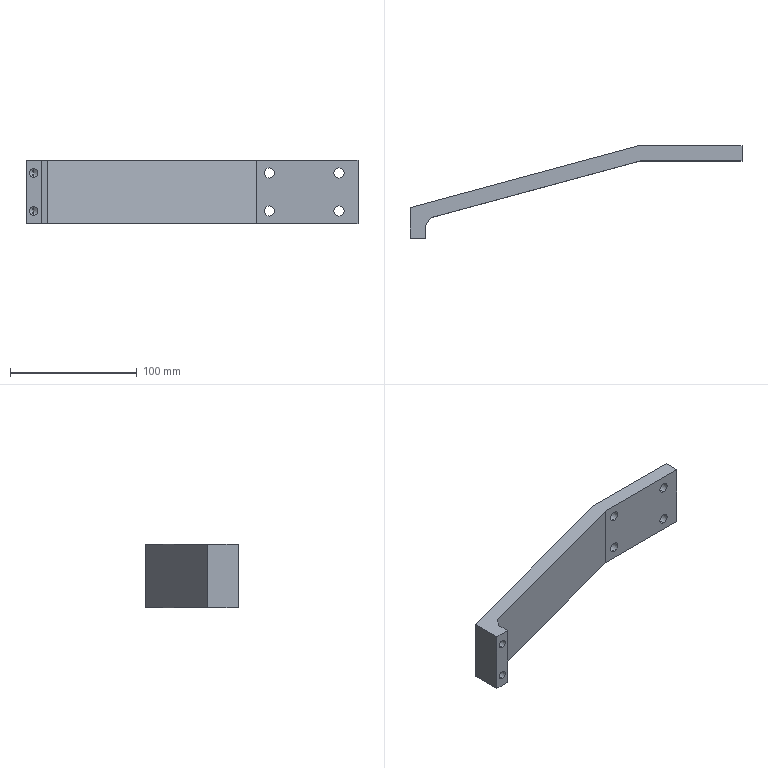Part | SolidWorks | features BaseBody 1 | 1 solid | 27 faces | box 262 x 73 x 50 mm | volume 166333 mm3 | cylinder 12 | plane 11 | cone 4 | commonest cylinder face diameters 8 x8 6.8 x4
STEP:
#1=CARTESIAN_POINT('',(260.,-92.,-78.879));
#2=VERTEX_POINT('',#1);
#3=CARTESIAN_POINT('',(260.,-92.,-86.879));
#4=VERTEX_POINT('',#3);
#5=CARTESIAN_POINT('',(260.,-92.,-82.879));
#6=DIRECTION('',(0.,-1.,0.));
#7=DIRECTION('',(0.,0.,1.));
#8=AXIS2_PLACEMENT_3D('',#5,#6,#7);
#9=CIRCLE('',#8,4.);
#10=EDGE_CURVE('',#2,#4,#9,.T.);
#11=ORIENTED_EDGE('',*,*,#10,.T.);
#12=CARTESIAN_POINT('',(260.,-80.,-86.879));
#13=VERTEX_POINT('',#12);
#14=CARTESIAN_POINT('',(260.,-153.,-86.879));
#15=DIRECTION('',(0.,1.,0.));
#16=VECTOR('',#15,1000.);
#17=LINE('',#14,#16);
#18=EDGE_CURVE('',#4,#13,#17,.T.);
#19=ORIENTED_EDGE('',*,*,#18,.T.);
#20=CARTESIAN_POINT('',(260.,-80.,-78.879));
#21=VERTEX_POINT('',#20);
#22=CARTESIAN_POINT('',(260.,-80.,-82.879));
#23=DIRECTION('',(0.,1.,0.));
#24=DIRECTION('',(0.,0.,1.));
#25=AXIS2_PLACEMENT_3D('',#22,#23,#24);
#26=CIRCLE('',#25,4.);
#27=EDGE_CURVE('',#13,#21,#26,.T.);
#28=ORIENTED_EDGE('',*,*,#27,.T.);
#29=CARTESIAN_POINT('',(260.,-153.,-78.879));
#30=DIRECTION('',(0.,1.,0.));
#31=VECTOR('',#30,1000.);
#32=LINE('',#29,#31);
#33=EDGE_CURVE('',#2,#21,#32,.T.);
#34=ORIENTED_EDGE('',*,*,#33,.F.);
#35=EDGE_LOOP('',(#11,#19,#28,#34));
#36=FACE_OUTER_BOUND('',#35,.T.);
#37=CARTESIAN_POINT('',(260.,-153.,-82.879));
#38=DIRECTION('',(0.,1.,0.));
#39=DIRECTION('',(0.,0.,1.));
#40=AXIS2_PLACEMENT_3D('',#37,#38,#39);
#41=CYLINDRICAL_SURFACE('',#40,4.);
#42=ADVANCED_FACE('',(#36),#41,.F.);
#43=CARTESIAN_POINT('',(260.,-92.,-48.879));
#44=VERTEX_POINT('',#43);
#45=CARTESIAN_POINT('',(260.,-92.,-56.879));
#46=VERTEX_POINT('',#45);
#47=CARTESIAN_POINT('',(260.,-92.,-52.879));
#48=DIRECTION('',(0.,-1.,0.));
#49=DIRECTION('',(0.,0.,1.));
#50=AXIS2_PLACEMENT_3D('',#47,#48,#49);
#51=CIRCLE('',#50,4.);
#52=EDGE_CURVE('',#44,#46,#51,.T.);
#53=ORIENTED_EDGE('',*,*,#52,.T.);
#54=CARTESIAN_POINT('',(260.,-80.,-56.879));
#55=VERTEX_POINT('',#54);
#56=CARTESIAN_POINT('',(260.,-153.,-56.879));
#57=DIRECTION('',(0.,1.,0.));
#58=VECTOR('',#57,1000.);
#59=LINE('',#56,#58);
#60=EDGE_CURVE('',#46,#55,#59,.T.);
#61=ORIENTED_EDGE('',*,*,#60,.T.);
#62=CARTESIAN_POINT('',(260.,-80.,-48.879));
#63=VERTEX_POINT('',#62);
#64=CARTESIAN_POINT('',(260.,-80.,-52.879));
#65=DIRECTION('',(0.,1.,0.));
#66=DIRECTION('',(0.,0.,1.));
#67=AXIS2_PLACEMENT_3D('',#64,#65,#66);
#68=CIRCLE('',#67,4.);
#69=EDGE_CURVE('',#55,#63,#68,.T.);
#70=ORIENTED_EDGE('',*,*,#69,.T.);
#71=CARTESIAN_POINT('',(260.,-153.,-48.879));
#72=DIRECTION('',(0.,1.,0.));
#73=VECTOR('',#72,1000.);
#74=LINE('',#71,#73);
#75=EDGE_CURVE('',#44,#63,#74,.T.);
#76=ORIENTED_EDGE('',*,*,#75,.F.);
#77=EDGE_LOOP('',(#53,#61,#70,#76));
#78=FACE_OUTER_BOUND('',#77,.T.);
#79=CARTESIAN_POINT('',(260.,-153.,-52.879));
#80=DIRECTION('',(0.,1.,0.));
#81=DIRECTION('',(0.,0.,1.));
#82=AXIS2_PLACEMENT_3D('',#79,#80,#81);
#83=CYLINDRICAL_SURFACE('',#82,4.);
#84=ADVANCED_FACE('',(#78),#83,.F.);
#85=CARTESIAN_POINT('',(315.,-92.,-48.879));
#86=VERTEX_POINT('',#85);
#87=CARTESIAN_POINT('',(315.,-92.,-56.879));
#88=VERTEX_POINT('',#87);
#89=CARTESIAN_POINT('',(315.,-92.,-52.879));
#90=DIRECTION('',(0.,-1.,0.));
#91=DIRECTION('',(0.,0.,1.));
#92=AXIS2_PLACEMENT_3D('',#89,#90,#91);
#93=CIRCLE('',#92,4.);
#94=EDGE_CURVE('',#86,#88,#93,.T.);
#95=ORIENTED_EDGE('',*,*,#94,.T.);
#96=CARTESIAN_POINT('',(315.,-80.,-56.879));
#97=VERTEX_POINT('',#96);
#98=CARTESIAN_POINT('',(315.,-153.,-56.879));
#99=DIRECTION('',(0.,1.,0.));
#100=VECTOR('',#99,1000.);
#101=LINE('',#98,#100);
#102=EDGE_CURVE('',#88,#97,#101,.T.);
#103=ORIENTED_EDGE('',*,*,#102,.T.);
#104=CARTESIAN_POINT('',(315.,-80.,-48.879));
#105=VERTEX_POINT('',#104);
#106=CARTESIAN_POINT('',(315.,-80.,-52.879));
#107=DIRECTION('',(0.,1.,0.));
#108=DIRECTION('',(0.,0.,1.));
#109=AXIS2_PLACEMENT_3D('',#106,#107,#108);
#110=CIRCLE('',#109,4.);
#111=EDGE_CURVE('',#97,#105,#110,.T.);
#112=ORIENTED_EDGE('',*,*,#111,.T.);
#113=CARTESIAN_POINT('',(315.,-153.,-48.879));
#114=DIRECTION('',(0.,1.,0.));
#115=VECTOR('',#114,1000.);
#116=LINE('',#113,#115);
#117=EDGE_CURVE('',#86,#105,#116,.T.);
#118=ORIENTED_EDGE('',*,*,#117,.F.);
#119=EDGE_LOOP('',(#95,#103,#112,#118));
#120=FACE_OUTER_BOUND('',#119,.T.);
#121=CARTESIAN_POINT('',(315.,-153.,-52.879));
#122=DIRECTION('',(0.,1.,0.));
#123=DIRECTION('',(0.,0.,1.));
#124=AXIS2_PLACEMENT_3D('',#121,#122,#123);
#125=CYLINDRICAL_SURFACE('',#124,4.);
#126=ADVANCED_FACE('',(#120),#125,.F.);
#127=CARTESIAN_POINT('',(315.,-92.,-78.879));
#128=VERTEX_POINT('',#127);
#129=CARTESIAN_POINT('',(315.,-92.,-86.879));
#130=VERTEX_POINT('',#129);
#131=CARTESIAN_POINT('',(315.,-92.,-82.879));
#132=DIRECTION('',(0.,-1.,0.));
#133=DIRECTION('',(0.,0.,1.));
#134=AXIS2_PLACEMENT_3D('',#131,#132,#133);
#135=CIRCLE('',#134,4.);
#136=EDGE_CURVE('',#128,#130,#135,.T.);
#137=ORIENTED_EDGE('',*,*,#136,.T.);
#138=CARTESIAN_POINT('',(315.,-80.,-86.879));
#139=VERTEX_POINT('',#138);
#140=CARTESIAN_POINT('',(315.,-153.,-86.879));
#141=DIRECTION('',(0.,1.,0.));
#142=VECTOR('',#141,1000.);
#143=LINE('',#140,#142);
#144=EDGE_CURVE('',#130,#139,#143,.T.);
#145=ORIENTED_EDGE('',*,*,#144,.T.);
#146=CARTESIAN_POINT('',(315.,-80.,-78.879));
#147=VERTEX_POINT('',#146);
#148=CARTESIAN_POINT('',(315.,-80.,-82.879));
#149=DIRECTION('',(0.,1.,0.));
#150=DIRECTION('',(0.,0.,1.));
#151=AXIS2_PLACEMENT_3D('',#148,#149,#150);
#152=CIRCLE('',#151,4.);
#153=EDGE_CURVE('',#139,#147,#152,.T.);
#154=ORIENTED_EDGE('',*,*,#153,.T.);
#155=CARTESIAN_POINT('',(315.,-153.,-78.879));
#156=DIRECTION('',(0.,1.,0.));
#157=VECTOR('',#156,1000.);
#158=LINE('',#155,#157);
#159=EDGE_CURVE('',#128,#147,#158,.T.);
#160=ORIENTED_EDGE('',*,*,#159,.F.);
#161=EDGE_LOOP('',(#137,#145,#154,#160));
#162=FACE_OUTER_BOUND('',#161,.T.);
#163=CARTESIAN_POINT('',(315.,-153.,-82.879));
#164=DIRECTION('',(0.,1.,0.));
#165=DIRECTION('',(0.,0.,1.));
#166=AXIS2_PLACEMENT_3D('',#163,#164,#165);
#167=CYLINDRICAL_SURFACE('',#166,4.);
#168=ADVANCED_FACE('',(#162),#167,.F.);
#169=CARTESIAN_POINT('',(74.,-140.,-49.479));
#170=VERTEX_POINT('',#169);
#171=CARTESIAN_POINT('',(74.,-140.,-56.279));
#172=VERTEX_POINT('',#171);
#173=CARTESIAN_POINT('',(74.,-140.,-52.879));
#174=DIRECTION('',(0.,-1.,0.));
#175=DIRECTION('',(0.,0.,-1.));
#176=AXIS2_PLACEMENT_3D('',#173,#174,#175);
#177=CIRCLE('',#176,3.4);
#178=EDGE_CURVE('',#170,#172,#177,.T.);
#179=ORIENTED_EDGE('',*,*,#178,.F.);
#180=CARTESIAN_POINT('',(74.,-153.,-49.479));
#181=VERTEX_POINT('',#180);
#182=CARTESIAN_POINT('',(74.,-153.,-49.479));
#183=DIRECTION('',(0.,-1.,0.));
#184=VECTOR('',#183,1000.);
#185=LINE('',#182,#184);
#186=EDGE_CURVE('',#170,#181,#185,.T.);
#187=ORIENTED_EDGE('',*,*,#186,.T.);
#188=CARTESIAN_POINT('',(74.,-153.,-56.279));
#189=VERTEX_POINT('',#188);
#190=CARTESIAN_POINT('',(74.,-153.,-52.879));
#191=DIRECTION('',(0.,-1.,0.));
#192=DIRECTION('',(0.,0.,-1.));
#193=AXIS2_PLACEMENT_3D('',#190,#191,#192);
#194=CIRCLE('',#193,3.4);
#195=EDGE_CURVE('',#181,#189,#194,.T.);
#196=ORIENTED_EDGE('',*,*,#195,.T.);
#197=CARTESIAN_POINT('',(74.,-153.,-56.279));
#198=DIRECTION('',(0.,-1.,0.));
#199=VECTOR('',#198,1000.);
#200=LINE('',#197,#199);
#201=EDGE_CURVE('',#172,#189,#200,.T.);
#202=ORIENTED_EDGE('',*,*,#201,.F.);
#203=EDGE_LOOP('',(#179,#187,#196,#202));
#204=FACE_OUTER_BOUND('',#203,.T.);
#205=CARTESIAN_POINT('',(74.,-153.,-52.879));
#206=DIRECTION('',(0.,-1.,0.));
#207=DIRECTION('',(0.,0.,-1.));
#208=AXIS2_PLACEMENT_3D('',#205,#206,#207);
#209=CYLINDRICAL_SURFACE('',#208,3.4);
#210=ADVANCED_FACE('',(#204),#209,.F.);
#211=CARTESIAN_POINT('',(74.,-140.,-79.479));
#212=VERTEX_POINT('',#211);
#213=CARTESIAN_POINT('',(74.,-140.,-86.279));
#214=VERTEX_POINT('',#213);
#215=CARTESIAN_POINT('',(74.,-140.,-82.879));
#216=DIRECTION('',(0.,-1.,0.));
#217=DIRECTION('',(0.,0.,-1.));
#218=AXIS2_PLACEMENT_3D('',#215,#216,#217);
#219=CIRCLE('',#218,3.4);
#220=EDGE_CURVE('',#212,#214,#219,.T.);
#221=ORIENTED_EDGE('',*,*,#220,.F.);
#222=CARTESIAN_POINT('',(74.,-153.,-79.479));
#223=VERTEX_POINT('',#222);
#224=CARTESIAN_POINT('',(74.,-153.,-79.479));
#225=DIRECTION('',(0.,-1.,0.));
#226=VECTOR('',#225,1000.);
#227=LINE('',#224,#226);
#228=EDGE_CURVE('',#212,#223,#227,.T.);
#229=ORIENTED_EDGE('',*,*,#228,.T.);
#230=CARTESIAN_POINT('',(74.,-153.,-86.279));
#231=VERTEX_POINT('',#230);
#232=CARTESIAN_POINT('',(74.,-153.,-82.879));
#233=DIRECTION('',(0.,-1.,0.));
#234=DIRECTION('',(0.,0.,-1.));
#235=AXIS2_PLACEMENT_3D('',#232,#233,#234);
#236=CIRCLE('',#235,3.4);
#237=EDGE_CURVE('',#223,#231,#236,.T.);
#238=ORIENTED_EDGE('',*,*,#237,.T.);
#239=CARTESIAN_POINT('',(74.,-153.,-86.279));
#240=DIRECTION('',(0.,-1.,0.));
#241=VECTOR('',#240,1000.);
#242=LINE('',#239,#241);
#243=EDGE_CURVE('',#214,#231,#242,.T.);
#244=ORIENTED_EDGE('',*,*,#243,.F.);
#245=EDGE_LOOP('',(#221,#229,#238,#244));
#246=FACE_OUTER_BOUND('',#245,.T.);
#247=CARTESIAN_POINT('',(74.,-153.,-82.879));
#248=DIRECTION('',(0.,-1.,0.));
#249=DIRECTION('',(0.,0.,-1.));
#250=AXIS2_PLACEMENT_3D('',#247,#248,#249);
#251=CYLINDRICAL_SURFACE('',#250,3.4);
#252=ADVANCED_FACE('',(#246),#251,.F.);
#253=CARTESIAN_POINT('',(74.,-137.957,-52.879));
#254=VERTEX_POINT('',#253);
#255=CARTESIAN_POINT('',(74.,-140.,-56.279));
#256=DIRECTION('',(0.,-0.515,-0.8572));
#257=VECTOR('',#256,1000.);
#258=LINE('',#255,#257);
#259=EDGE_CURVE('',#254,#172,#258,.T.);
#260=ORIENTED_EDGE('',*,*,#259,.F.);
#261=CARTESIAN_POINT('',(74.,-140.,-49.479));
#262=DIRECTION('',(0.,-0.515,0.8572));
#263=VECTOR('',#262,1000.);
#264=LINE('',#261,#263);
#265=EDGE_CURVE('',#254,#170,#264,.T.);
#266=ORIENTED_EDGE('',*,*,#265,.T.);
#267=ORIENTED_EDGE('',*,*,#178,.T.);
#268=EDGE_LOOP('',(#260,#266,#267));
#269=FACE_OUTER_BOUND('',#268,.T.);
#270=CARTESIAN_POINT('',(74.,-140.,-52.879));
#271=DIRECTION('',(0.,-1.,0.));
#272=DIRECTION('',(0.,0.,-1.));
#273=AXIS2_PLACEMENT_3D('',#270,#271,#272);
#274=CONICAL_SURFACE('',#273,3.4,1.03);
#275=ADVANCED_FACE('',(#269),#274,.F.);
#276=CARTESIAN_POINT('',(74.,-137.957,-82.879));
#277=VERTEX_POINT('',#276);
#278=CARTESIAN_POINT('',(74.,-140.,-86.279));
#279=DIRECTION('',(0.,-0.515,-0.8572));
#280=VECTOR('',#279,1000.);
#281=LINE('',#278,#280);
#282=EDGE_CURVE('',#277,#214,#281,.T.);
#283=ORIENTED_EDGE('',*,*,#282,.F.);
#284=CARTESIAN_POINT('',(74.,-140.,-79.479));
#285=DIRECTION('',(0.,-0.515,0.8572));
#286=VECTOR('',#285,1000.);
#287=LINE('',#284,#286);
#288=EDGE_CURVE('',#277,#212,#287,.T.);
#289=ORIENTED_EDGE('',*,*,#288,.T.);
#290=ORIENTED_EDGE('',*,*,#220,.T.);
#291=EDGE_LOOP('',(#283,#289,#290));
#292=FACE_OUTER_BOUND('',#291,.T.);
#293=CARTESIAN_POINT('',(74.,-140.,-82.879));
#294=DIRECTION('',(0.,-1.,0.));
#295=DIRECTION('',(0.,0.,-1.));
#296=AXIS2_PLACEMENT_3D('',#293,#294,#295);
#297=CONICAL_SURFACE('',#296,3.4,1.03);
#298=ADVANCED_FACE('',(#292),#297,.F.);
#299=CARTESIAN_POINT('',(248.405,-80.,-92.879));
#300=VERTEX_POINT('',#299);
#301=CARTESIAN_POINT('',(248.405,-80.,-42.879));
#302=VERTEX_POINT('',#301);
#303=CARTESIAN_POINT('',(248.405,-80.,-92.879));
#304=DIRECTION('',(0.,0.,1.));
#305=VECTOR('',#304,1000.);
#306=LINE('',#303,#305);
#307=EDGE_CURVE('',#300,#302,#306,.T.);
#308=ORIENTED_EDGE('',*,*,#307,.F.);
#309=CARTESIAN_POINT('',(68.,-128.816,-92.879));
#310=VERTEX_POINT('',#309);
#311=CARTESIAN_POINT('',(68.,-128.816,-92.879));
#312=DIRECTION('',(0.9653,0.2612,0.));
#313=VECTOR('',#312,1000.);
#314=LINE('',#311,#313);
#315=EDGE_CURVE('',#310,#300,#314,.T.);
#316=ORIENTED_EDGE('',*,*,#315,.F.);
#317=CARTESIAN_POINT('',(68.,-128.816,-42.879));
#318=VERTEX_POINT('',#317);
#319=CARTESIAN_POINT('',(68.,-128.816,-92.879));
#320=DIRECTION('',(0.,0.,-1.));
#321=VECTOR('',#320,1000.);
#322=LINE('',#319,#321);
#323=EDGE_CURVE('',#318,#310,#322,.T.);
#324=ORIENTED_EDGE('',*,*,#323,.F.);
#325=CARTESIAN_POINT('',(68.,-128.816,-42.879));
#326=DIRECTION('',(-0.9653,-0.2612,0.));
#327=VECTOR('',#326,1000.);
#328=LINE('',#325,#327);
#329=EDGE_CURVE('',#302,#318,#328,.T.);
#330=ORIENTED_EDGE('',*,*,#329,.F.);
#331=EDGE_LOOP('',(#308,#316,#324,#330));
#332=FACE_OUTER_BOUND('',#331,.T.);
#333=CARTESIAN_POINT('',(68.,-128.816,-92.879));
#334=DIRECTION('',(0.2612,-0.9653,0.));
#335=DIRECTION('',(0.9653,0.2612,0.));
#336=AXIS2_PLACEMENT_3D('',#333,#334,#335);
#337=PLANE('',#336);
#338=ADVANCED_FACE('',(#332),#337,.F.);
#339=CARTESIAN_POINT('',(80.,-143.,-42.879));
#340=VERTEX_POINT('',#339);
#341=CARTESIAN_POINT('',(80.,-153.,-42.879));
#342=VERTEX_POINT('',#341);
#343=CARTESIAN_POINT('',(80.,-108.6,-42.879));
#344=DIRECTION('',(0.,-1.,0.));
#345=VECTOR('',#344,1000.);
#346=LINE('',#343,#345);
#347=EDGE_CURVE('',#340,#342,#346,.T.);
#348=ORIENTED_EDGE('',*,*,#347,.F.);
#349=CARTESIAN_POINT('',(84.826,-136.694,-42.879));
#350=VERTEX_POINT('',#349);
#351=CARTESIAN_POINT('',(84.826,-136.694,-42.879));
#352=DIRECTION('',(-0.6078,-0.7941,0.));
#353=VECTOR('',#352,1000.);
#354=LINE('',#351,#353);
#355=EDGE_CURVE('',#350,#340,#354,.T.);
#356=ORIENTED_EDGE('',*,*,#355,.F.);
#357=CARTESIAN_POINT('',(250.,-92.,-42.879));
#358=VERTEX_POINT('',#357);
#359=CARTESIAN_POINT('',(250.,-92.,-42.879));
#360=DIRECTION('',(-0.9653,-0.2612,0.));
#361=VECTOR('',#360,1000.);
#362=LINE('',#359,#361);
#363=EDGE_CURVE('',#358,#350,#362,.T.);
#364=ORIENTED_EDGE('',*,*,#363,.F.);
#365=CARTESIAN_POINT('',(330.,-92.,-42.879));
#366=VERTEX_POINT('',#365);
#367=CARTESIAN_POINT('',(68.,-92.,-42.879));
#368=DIRECTION('',(-1.,0.,0.));
#369=VECTOR('',#368,1000.);
#370=LINE('',#367,#369);
#371=EDGE_CURVE('',#366,#358,#370,.T.);
#372=ORIENTED_EDGE('',*,*,#371,.F.);
#373=CARTESIAN_POINT('',(330.,-80.,-42.879));
#374=VERTEX_POINT('',#373);
#375=CARTESIAN_POINT('',(330.,-108.6,-42.879));
#376=DIRECTION('',(0.,-1.,0.));
#377=VECTOR('',#376,1000.);
#378=LINE('',#375,#377);
#379=EDGE_CURVE('',#374,#366,#378,.T.);
#380=ORIENTED_EDGE('',*,*,#379,.F.);
#381=CARTESIAN_POINT('',(68.,-80.,-42.879));
#382=DIRECTION('',(1.,0.,0.));
#383=VECTOR('',#382,1000.);
#384=LINE('',#381,#383);
#385=EDGE_CURVE('',#302,#374,#384,.T.);
#386=ORIENTED_EDGE('',*,*,#385,.F.);
#387=ORIENTED_EDGE('',*,*,#329,.T.);
#388=CARTESIAN_POINT('',(68.,-153.,-42.879));
#389=VERTEX_POINT('',#388);
#390=CARTESIAN_POINT('',(68.,-108.6,-42.879));
#391=DIRECTION('',(0.,1.,0.));
#392=VECTOR('',#391,1000.);
#393=LINE('',#390,#392);
#394=EDGE_CURVE('',#389,#318,#393,.T.);
#395=ORIENTED_EDGE('',*,*,#394,.F.);
#396=CARTESIAN_POINT('',(68.,-153.,-42.879));
#397=DIRECTION('',(-1.,0.,0.));
#398=VECTOR('',#397,1000.);
#399=LINE('',#396,#398);
#400=EDGE_CURVE('',#342,#389,#399,.T.);
#401=ORIENTED_EDGE('',*,*,#400,.F.);
#402=EDGE_LOOP('',(#348,#356,#364,#372,#380,#386,#387,#395,#401));
#403=FACE_OUTER_BOUND('',#402,.T.);
#404=CARTESIAN_POINT('',(68.,-108.6,-42.879));
#405=DIRECTION('',(0.,0.,-1.));
#406=DIRECTION('',(-1.,0.,0.));
#407=AXIS2_PLACEMENT_3D('',#404,#405,#406);
#408=PLANE('',#407);
#409=ADVANCED_FACE('',(#403),#408,.F.);
#410=CARTESIAN_POINT('',(330.,-80.,-92.879));
#411=VERTEX_POINT('',#410);
#412=CARTESIAN_POINT('',(330.,-80.,-92.879));
#413=DIRECTION('',(0.,0.,1.));
#414=VECTOR('',#413,1000.);
#415=LINE('',#412,#414);
#416=EDGE_CURVE('',#411,#374,#415,.T.);
#417=ORIENTED_EDGE('',*,*,#416,.F.);
#418=CARTESIAN_POINT('',(248.405,-80.,-92.879));
#419=DIRECTION('',(1.,0.,0.));
#420=VECTOR('',#419,1000.);
#421=LINE('',#418,#420);
#422=EDGE_CURVE('',#300,#411,#421,.T.);
#423=ORIENTED_EDGE('',*,*,#422,.F.);
#424=ORIENTED_EDGE('',*,*,#307,.T.);
#425=ORIENTED_EDGE('',*,*,#385,.T.);
#426=EDGE_LOOP('',(#417,#423,#424,#425));
#427=FACE_OUTER_BOUND('',#426,.T.);
#428=CARTESIAN_POINT('',(260.,-80.,-82.879));
#429=DIRECTION('',(0.,1.,0.));
#430=DIRECTION('',(0.,0.,1.));
#431=AXIS2_PLACEMENT_3D('',#428,#429,#430);
#432=CIRCLE('',#431,4.);
#433=EDGE_CURVE('',#21,#13,#432,.T.);
#434=ORIENTED_EDGE('',*,*,#433,.F.);
#435=ORIENTED_EDGE('',*,*,#27,.F.);
#436=EDGE_LOOP('',(#434,#435));
#437=FACE_BOUND('',#436,.T.);
#438=CARTESIAN_POINT('',(260.,-80.,-52.879));
#439=DIRECTION('',(0.,1.,0.));
#440=DIRECTION('',(0.,0.,1.));
#441=AXIS2_PLACEMENT_3D('',#438,#439,#440);
#442=CIRCLE('',#441,4.);
#443=EDGE_CURVE('',#63,#55,#442,.T.);
#444=ORIENTED_EDGE('',*,*,#443,.F.);
#445=ORIENTED_EDGE('',*,*,#69,.F.);
#446=EDGE_LOOP('',(#444,#445));
#447=FACE_BOUND('',#446,.T.);
#448=CARTESIAN_POINT('',(315.,-80.,-52.879));
#449=DIRECTION('',(0.,1.,0.));
#450=DIRECTION('',(0.,0.,1.));
#451=AXIS2_PLACEMENT_3D('',#448,#449,#450);
#452=CIRCLE('',#451,4.);
#453=EDGE_CURVE('',#105,#97,#452,.T.);
#454=ORIENTED_EDGE('',*,*,#453,.F.);
#455=ORIENTED_EDGE('',*,*,#111,.F.);
#456=EDGE_LOOP('',(#454,#455));
#457=FACE_BOUND('',#456,.T.);
#458=CARTESIAN_POINT('',(315.,-80.,-82.879));
#459=DIRECTION('',(0.,1.,0.));
#460=DIRECTION('',(0.,0.,1.));
#461=AXIS2_PLACEMENT_3D('',#458,#459,#460);
#462=CIRCLE('',#461,4.);
#463=EDGE_CURVE('',#147,#139,#462,.T.);
#464=ORIENTED_EDGE('',*,*,#463,.F.);
#465=ORIENTED_EDGE('',*,*,#153,.F.);
#466=EDGE_LOOP('',(#464,#465));
#467=FACE_BOUND('',#466,.T.);
#468=CARTESIAN_POINT('',(248.405,-80.,-92.879));
#469=DIRECTION('',(0.,-1.,0.));
#470=DIRECTION('',(0.,0.,-1.));
#471=AXIS2_PLACEMENT_3D('',#468,#469,#470);
#472=PLANE('',#471);
#473=ADVANCED_FACE('',(#427,#437,#447,#457,#467),#472,.F.);
#474=CARTESIAN_POINT('',(84.826,-136.694,-92.879));
#475=VERTEX_POINT('',#474);
#476=CARTESIAN_POINT('',(80.,-143.,-92.879));
#477=VERTEX_POINT('',#476);
#478=CARTESIAN_POINT('',(84.826,-136.694,-92.879));
#479=DIRECTION('',(-0.6078,-0.7941,0.));
#480=VECTOR('',#479,1000.);
#481=LINE('',#478,#480);
#482=EDGE_CURVE('',#475,#477,#481,.T.);
#483=ORIENTED_EDGE('',*,*,#482,.T.);
#484=CARTESIAN_POINT('',(80.,-153.,-92.879));
#485=VERTEX_POINT('',#484);
#486=CARTESIAN_POINT('',(80.,-108.6,-92.879));
#487=DIRECTION('',(0.,-1.,0.));
#488=VECTOR('',#487,1000.);
#489=LINE('',#486,#488);
#490=EDGE_CURVE('',#477,#485,#489,.T.);
#491=ORIENTED_EDGE('',*,*,#490,.T.);
#492=CARTESIAN_POINT('',(68.,-153.,-92.879));
#493=VERTEX_POINT('',#492);
#494=CARTESIAN_POINT('',(68.,-153.,-92.879));
#495=DIRECTION('',(-1.,0.,0.));
#496=VECTOR('',#495,1000.);
#497=LINE('',#494,#496);
#498=EDGE_CURVE('',#485,#493,#497,.T.);
#499=ORIENTED_EDGE('',*,*,#498,.T.);
#500=CARTESIAN_POINT('',(68.,-108.6,-92.879));
#501=DIRECTION('',(0.,1.,0.));
#502=VECTOR('',#501,1000.);
#503=LINE('',#500,#502);
#504=EDGE_CURVE('',#493,#310,#503,.T.);
#505=ORIENTED_EDGE('',*,*,#504,.T.);
#506=ORIENTED_EDGE('',*,*,#315,.T.);
#507=ORIENTED_EDGE('',*,*,#422,.T.);
#508=CARTESIAN_POINT('',(330.,-92.,-92.879));
#509=VERTEX_POINT('',#508);
#510=CARTESIAN_POINT('',(330.,-108.6,-92.879));
#511=DIRECTION('',(0.,-1.,0.));
#512=VECTOR('',#511,1000.);
#513=LINE('',#510,#512);
#514=EDGE_CURVE('',#411,#509,#513,.T.);
#515=ORIENTED_EDGE('',*,*,#514,.T.);
#516=CARTESIAN_POINT('',(250.,-92.,-92.879));
#517=VERTEX_POINT('',#516);
#518=CARTESIAN_POINT('',(68.,-92.,-92.879));
#519=DIRECTION('',(-1.,0.,0.));
#520=VECTOR('',#519,1000.);
#521=LINE('',#518,#520);
#522=EDGE_CURVE('',#509,#517,#521,.T.);
#523=ORIENTED_EDGE('',*,*,#522,.T.);
#524=CARTESIAN_POINT('',(250.,-92.,-92.879));
#525=DIRECTION('',(-0.9653,-0.2612,0.));
#526=VECTOR('',#525,1000.);
#527=LINE('',#524,#526);
#528=EDGE_CURVE('',#517,#475,#527,.T.);
#529=ORIENTED_EDGE('',*,*,#528,.T.);
#530=EDGE_LOOP('',(#483,#491,#499,#505,#506,#507,#515,#523,#529));
#531=FACE_OUTER_BOUND('',#530,.T.);
#532=CARTESIAN_POINT('',(68.,-108.6,-92.879));
#533=DIRECTION('',(0.,0.,-1.));
#534=DIRECTION('',(-1.,0.,0.));
#535=AXIS2_PLACEMENT_3D('',#532,#533,#534);
#536=PLANE('',#535);
#537=ADVANCED_FACE('',(#531),#536,.T.);
#538=ORIENTED_EDGE('',*,*,#323,.T.);
#539=ORIENTED_EDGE('',*,*,#504,.F.);
#540=CARTESIAN_POINT('',(68.,-153.,-92.879));
#541=DIRECTION('',(0.,0.,-1.));
#542=VECTOR('',#541,1000.);
#543=LINE('',#540,#542);
#544=EDGE_CURVE('',#389,#493,#543,.T.);
#545=ORIENTED_EDGE('',*,*,#544,.F.);
#546=ORIENTED_EDGE('',*,*,#394,.T.);
#547=EDGE_LOOP('',(#538,#539,#545,#546));
#548=FACE_OUTER_BOUND('',#547,.T.);
#549=CARTESIAN_POINT('',(68.,-153.,-92.879));
#550=DIRECTION('',(1.,0.,0.));
#551=DIRECTION('',(0.,0.,-1.));
#552=AXIS2_PLACEMENT_3D('',#549,#550,#551);
#553=PLANE('',#552);
#554=ADVANCED_FACE('',(#548),#553,.F.);
#555=ORIENTED_EDGE('',*,*,#544,.T.);
#556=ORIENTED_EDGE('',*,*,#498,.F.);
#557=CARTESIAN_POINT('',(80.,-153.,-92.879));
#558=DIRECTION('',(0.,0.,-1.));
#559=VECTOR('',#558,1000.);
#560=LINE('',#557,#559);
#561=EDGE_CURVE('',#342,#485,#560,.T.);
#562=ORIENTED_EDGE('',*,*,#561,.F.);
#563=ORIENTED_EDGE('',*,*,#400,.T.);
#564=EDGE_LOOP('',(#555,#556,#562,#563));
#565=FACE_OUTER_BOUND('',#564,.T.);
#566=CARTESIAN_POINT('',(74.,-153.,-52.879));
#567=DIRECTION('',(0.,-1.,0.));
#568=DIRECTION('',(0.,0.,-1.));
#569=AXIS2_PLACEMENT_3D('',#566,#567,#568);
#570=CIRCLE('',#569,3.4);
#571=EDGE_CURVE('',#189,#181,#570,.T.);
#572=ORIENTED_EDGE('',*,*,#571,.F.);
#573=ORIENTED_EDGE('',*,*,#195,.F.);
#574=EDGE_LOOP('',(#572,#573));
#575=FACE_BOUND('',#574,.T.);
#576=CARTESIAN_POINT('',(74.,-153.,-82.879));
#577=DIRECTION('',(0.,-1.,0.));
#578=DIRECTION('',(0.,0.,-1.));
#579=AXIS2_PLACEMENT_3D('',#576,#577,#578);
#580=CIRCLE('',#579,3.4);
#581=EDGE_CURVE('',#231,#223,#580,.T.);
#582=ORIENTED_EDGE('',*,*,#581,.F.);
#583=ORIENTED_EDGE('',*,*,#237,.F.);
#584=EDGE_LOOP('',(#582,#583));
#585=FACE_BOUND('',#584,.T.);
#586=CARTESIAN_POINT('',(80.,-153.,-92.879));
#587=DIRECTION('',(0.,1.,0.));
#588=DIRECTION('',(0.,0.,1.));
#589=AXIS2_PLACEMENT_3D('',#586,#587,#588);
#590=PLANE('',#589);
#591=ADVANCED_FACE('',(#565,#575,#585),#590,.F.);
#592=CARTESIAN_POINT('',(80.,-143.,-92.879));
#593=DIRECTION('',(0.,0.,-1.));
#594=VECTOR('',#593,1000.);
#595=LINE('',#592,#594);
#596=EDGE_CURVE('',#340,#477,#595,.T.);
#597=ORIENTED_EDGE('',*,*,#596,.F.);
#598=ORIENTED_EDGE('',*,*,#347,.T.);
#599=ORIENTED_EDGE('',*,*,#561,.T.);
#600=ORIENTED_EDGE('',*,*,#490,.F.);
#601=EDGE_LOOP('',(#597,#598,#599,#600));
#602=FACE_OUTER_BOUND('',#601,.T.);
#603=CARTESIAN_POINT('',(80.,-153.,-92.879));
#604=DIRECTION('',(-1.,0.,0.));
#605=DIRECTION('',(0.,0.,1.));
#606=AXIS2_PLACEMENT_3D('',#603,#604,#605);
#607=PLANE('',#606);
#608=ADVANCED_FACE('',(#602),#607,.F.);
#609=ORIENTED_EDGE('',*,*,#355,.T.);
#610=ORIENTED_EDGE('',*,*,#596,.T.);
#611=ORIENTED_EDGE('',*,*,#482,.F.);
#612=CARTESIAN_POINT('',(84.826,-136.694,-92.879));
#613=DIRECTION('',(0.,0.,1.));
#614=VECTOR('',#613,1000.);
#615=LINE('',#612,#614);
#616=EDGE_CURVE('',#475,#350,#615,.T.);
#617=ORIENTED_EDGE('',*,*,#616,.T.);
#618=EDGE_LOOP('',(#609,#610,#611,#617));
#619=FACE_OUTER_BOUND('',#618,.T.);
#620=CARTESIAN_POINT('',(80.,-143.,-92.879));
#621=DIRECTION('',(0.7941,-0.6078,0.));
#622=DIRECTION('',(0.6078,0.7941,0.));
#623=AXIS2_PLACEMENT_3D('',#620,#621,#622);
#624=PLANE('',#623);
#625=ADVANCED_FACE('',(#619),#624,.T.);
#626=ORIENTED_EDGE('',*,*,#616,.F.);
#627=ORIENTED_EDGE('',*,*,#528,.F.);
#628=CARTESIAN_POINT('',(250.,-92.,-92.879));
#629=DIRECTION('',(0.,0.,-1.));
#630=VECTOR('',#629,1000.);
#631=LINE('',#628,#630);
#632=EDGE_CURVE('',#358,#517,#631,.T.);
#633=ORIENTED_EDGE('',*,*,#632,.F.);
#634=ORIENTED_EDGE('',*,*,#363,.T.);
#635=EDGE_LOOP('',(#626,#627,#633,#634));
#636=FACE_OUTER_BOUND('',#635,.T.);
#637=CARTESIAN_POINT('',(80.,-138.,-92.879));
#638=DIRECTION('',(-0.2612,0.9653,0.));
#639=DIRECTION('',(-0.9653,-0.2612,0.));
#640=AXIS2_PLACEMENT_3D('',#637,#638,#639);
#641=PLANE('',#640);
#642=ADVANCED_FACE('',(#636),#641,.F.);
#643=ORIENTED_EDGE('',*,*,#632,.T.);
#644=ORIENTED_EDGE('',*,*,#522,.F.);
#645=CARTESIAN_POINT('',(330.,-92.,-92.879));
#646=DIRECTION('',(0.,0.,-1.));
#647=VECTOR('',#646,1000.);
#648=LINE('',#645,#647);
#649=EDGE_CURVE('',#366,#509,#648,.T.);
#650=ORIENTED_EDGE('',*,*,#649,.F.);
#651=ORIENTED_EDGE('',*,*,#371,.T.);
#652=EDGE_LOOP('',(#643,#644,#650,#651));
#653=FACE_OUTER_BOUND('',#652,.T.);
#654=ORIENTED_EDGE('',*,*,#10,.F.);
#655=CARTESIAN_POINT('',(260.,-92.,-82.879));
#656=DIRECTION('',(0.,-1.,0.));
#657=DIRECTION('',(0.,0.,1.));
#658=AXIS2_PLACEMENT_3D('',#655,#656,#657);
#659=CIRCLE('',#658,4.);
#660=EDGE_CURVE('',#4,#2,#659,.T.);
#661=ORIENTED_EDGE('',*,*,#660,.F.);
#662=EDGE_LOOP('',(#654,#661));
#663=FACE_BOUND('',#662,.T.);
#664=ORIENTED_EDGE('',*,*,#52,.F.);
#665=CARTESIAN_POINT('',(260.,-92.,-52.879));
#666=DIRECTION('',(0.,-1.,0.));
#667=DIRECTION('',(0.,0.,1.));
#668=AXIS2_PLACEMENT_3D('',#665,#666,#667);
#669=CIRCLE('',#668,4.);
#670=EDGE_CURVE('',#46,#44,#669,.T.);
#671=ORIENTED_EDGE('',*,*,#670,.F.);
#672=EDGE_LOOP('',(#664,#671));
#673=FACE_BOUND('',#672,.T.);
#674=ORIENTED_EDGE('',*,*,#94,.F.);
#675=CARTESIAN_POINT('',(315.,-92.,-52.879));
#676=DIRECTION('',(0.,-1.,0.));
#677=DIRECTION('',(0.,0.,1.));
#678=AXIS2_PLACEMENT_3D('',#675,#676,#677);
#679=CIRCLE('',#678,4.);
#680=EDGE_CURVE('',#88,#86,#679,.T.);
#681=ORIENTED_EDGE('',*,*,#680,.F.);
#682=EDGE_LOOP('',(#674,#681));
#683=FACE_BOUND('',#682,.T.);
#684=ORIENTED_EDGE('',*,*,#136,.F.);
#685=CARTESIAN_POINT('',(315.,-92.,-82.879));
#686=DIRECTION('',(0.,-1.,0.));
#687=DIRECTION('',(0.,0.,1.));
#688=AXIS2_PLACEMENT_3D('',#685,#686,#687);
#689=CIRCLE('',#688,4.);
#690=EDGE_CURVE('',#130,#128,#689,.T.);
#691=ORIENTED_EDGE('',*,*,#690,.F.);
#692=EDGE_LOOP('',(#684,#691));
#693=FACE_BOUND('',#692,.T.);
#694=CARTESIAN_POINT('',(250.,-92.,-92.879));
#695=DIRECTION('',(0.,1.,0.));
#696=DIRECTION('',(0.,0.,1.));
#697=AXIS2_PLACEMENT_3D('',#694,#695,#696);
#698=PLANE('',#697);
#699=ADVANCED_FACE('',(#653,#663,#673,#683,#693),#698,.F.);
#700=ORIENTED_EDGE('',*,*,#649,.T.);
#701=ORIENTED_EDGE('',*,*,#514,.F.);
#702=ORIENTED_EDGE('',*,*,#416,.T.);
#703=ORIENTED_EDGE('',*,*,#379,.T.);
#704=EDGE_LOOP('',(#700,#701,#702,#703));
#705=FACE_OUTER_BOUND('',#704,.T.);
#706=CARTESIAN_POINT('',(330.,-80.,-92.879));
#707=DIRECTION('',(-1.,0.,0.));
#708=DIRECTION('',(0.,0.,1.));
#709=AXIS2_PLACEMENT_3D('',#706,#707,#708);
#710=PLANE('',#709);
#711=ADVANCED_FACE('',(#705),#710,.F.);
#712=ORIENTED_EDGE('',*,*,#18,.F.);
#713=ORIENTED_EDGE('',*,*,#660,.T.);
#714=ORIENTED_EDGE('',*,*,#33,.T.);
#715=ORIENTED_EDGE('',*,*,#433,.T.);
#716=EDGE_LOOP('',(#712,#713,#714,#715));
#717=FACE_OUTER_BOUND('',#716,.T.);
#718=CARTESIAN_POINT('',(260.,-153.,-82.879));
#719=DIRECTION('',(0.,1.,0.));
#720=DIRECTION('',(0.,0.,1.));
#721=AXIS2_PLACEMENT_3D('',#718,#719,#720);
#722=CYLINDRICAL_SURFACE('',#721,4.);
#723=ADVANCED_FACE('',(#717),#722,.F.);
#724=ORIENTED_EDGE('',*,*,#60,.F.);
#725=ORIENTED_EDGE('',*,*,#670,.T.);
#726=ORIENTED_EDGE('',*,*,#75,.T.);
#727=ORIENTED_EDGE('',*,*,#443,.T.);
#728=EDGE_LOOP('',(#724,#725,#726,#727));
#729=FACE_OUTER_BOUND('',#728,.T.);
#730=CARTESIAN_POINT('',(260.,-153.,-52.879));
#731=DIRECTION('',(0.,1.,0.));
#732=DIRECTION('',(0.,0.,1.));
#733=AXIS2_PLACEMENT_3D('',#730,#731,#732);
#734=CYLINDRICAL_SURFACE('',#733,4.);
#735=ADVANCED_FACE('',(#729),#734,.F.);
#736=ORIENTED_EDGE('',*,*,#102,.F.);
#737=ORIENTED_EDGE('',*,*,#680,.T.);
#738=ORIENTED_EDGE('',*,*,#117,.T.);
#739=ORIENTED_EDGE('',*,*,#453,.T.);
#740=EDGE_LOOP('',(#736,#737,#738,#739));
#741=FACE_OUTER_BOUND('',#740,.T.);
#742=CARTESIAN_POINT('',(315.,-153.,-52.879));
#743=DIRECTION('',(0.,1.,0.));
#744=DIRECTION('',(0.,0.,1.));
#745=AXIS2_PLACEMENT_3D('',#742,#743,#744);
#746=CYLINDRICAL_SURFACE('',#745,4.);
#747=ADVANCED_FACE('',(#741),#746,.F.);
#748=ORIENTED_EDGE('',*,*,#144,.F.);
#749=ORIENTED_EDGE('',*,*,#690,.T.);
#750=ORIENTED_EDGE('',*,*,#159,.T.);
#751=ORIENTED_EDGE('',*,*,#463,.T.);
#752=EDGE_LOOP('',(#748,#749,#750,#751));
#753=FACE_OUTER_BOUND('',#752,.T.);
#754=CARTESIAN_POINT('',(315.,-153.,-82.879));
#755=DIRECTION('',(0.,1.,0.));
#756=DIRECTION('',(0.,0.,1.));
#757=AXIS2_PLACEMENT_3D('',#754,#755,#756);
#758=CYLINDRICAL_SURFACE('',#757,4.);
#759=ADVANCED_FACE('',(#753),#758,.F.);
#760=ORIENTED_EDGE('',*,*,#186,.F.);
#761=CARTESIAN_POINT('',(74.,-140.,-52.879));
#762=DIRECTION('',(0.,-1.,0.));
#763=DIRECTION('',(0.,0.,-1.));
#764=AXIS2_PLACEMENT_3D('',#761,#762,#763);
#765=CIRCLE('',#764,3.4);
#766=EDGE_CURVE('',#172,#170,#765,.T.);
#767=ORIENTED_EDGE('',*,*,#766,.F.);
#768=ORIENTED_EDGE('',*,*,#201,.T.);
#769=ORIENTED_EDGE('',*,*,#571,.T.);
#770=EDGE_LOOP('',(#760,#767,#768,#769));
#771=FACE_OUTER_BOUND('',#770,.T.);
#772=CARTESIAN_POINT('',(74.,-153.,-52.879));
#773=DIRECTION('',(0.,-1.,0.));
#774=DIRECTION('',(0.,0.,-1.));
#775=AXIS2_PLACEMENT_3D('',#772,#773,#774);
#776=CYLINDRICAL_SURFACE('',#775,3.4);
#777=ADVANCED_FACE('',(#771),#776,.F.);
#778=ORIENTED_EDGE('',*,*,#228,.F.);
#779=CARTESIAN_POINT('',(74.,-140.,-82.879));
#780=DIRECTION('',(0.,-1.,0.));
#781=DIRECTION('',(0.,0.,-1.));
#782=AXIS2_PLACEMENT_3D('',#779,#780,#781);
#783=CIRCLE('',#782,3.4);
#784=EDGE_CURVE('',#214,#212,#783,.T.);
#785=ORIENTED_EDGE('',*,*,#784,.F.);
#786=ORIENTED_EDGE('',*,*,#243,.T.);
#787=ORIENTED_EDGE('',*,*,#581,.T.);
#788=EDGE_LOOP('',(#778,#785,#786,#787));
#789=FACE_OUTER_BOUND('',#788,.T.);
#790=CARTESIAN_POINT('',(74.,-153.,-82.879));
#791=DIRECTION('',(0.,-1.,0.));
#792=DIRECTION('',(0.,0.,-1.));
#793=AXIS2_PLACEMENT_3D('',#790,#791,#792);
#794=CYLINDRICAL_SURFACE('',#793,3.4);
#795=ADVANCED_FACE('',(#789),#794,.F.);
#796=ORIENTED_EDGE('',*,*,#265,.F.);
#797=ORIENTED_EDGE('',*,*,#259,.T.);
#798=ORIENTED_EDGE('',*,*,#766,.T.);
#799=EDGE_LOOP('',(#796,#797,#798));
#800=FACE_OUTER_BOUND('',#799,.T.);
#801=CARTESIAN_POINT('',(74.,-140.,-52.879));
#802=DIRECTION('',(0.,-1.,0.));
#803=DIRECTION('',(0.,0.,-1.));
#804=AXIS2_PLACEMENT_3D('',#801,#802,#803);
#805=CONICAL_SURFACE('',#804,3.4,1.03);
#806=ADVANCED_FACE('',(#800),#805,.F.);
#807=ORIENTED_EDGE('',*,*,#288,.F.);
#808=ORIENTED_EDGE('',*,*,#282,.T.);
#809=ORIENTED_EDGE('',*,*,#784,.T.);
#810=EDGE_LOOP('',(#807,#808,#809));
#811=FACE_OUTER_BOUND('',#810,.T.);
#812=CARTESIAN_POINT('',(74.,-140.,-82.879));
#813=DIRECTION('',(0.,-1.,0.));
#814=DIRECTION('',(0.,0.,-1.));
#815=AXIS2_PLACEMENT_3D('',#812,#813,#814);
#816=CONICAL_SURFACE('',#815,3.4,1.03);
#817=ADVANCED_FACE('',(#811),#816,.F.);
#818=CLOSED_SHELL('',(#42,#84,#126,#168,#210,#252,#275,#298,#338,#409,#473,#537,#554,#591,#608,#625,#642,#699,#711,#723,#735,#747,#759,#777,#795,#806,#817));
#819=MANIFOLD_SOLID_BREP('',#818);
#820=CARTESIAN_POINT('',(0.,0.,0.));
#821=DIRECTION('',(0.,0.,1.));
#822=DIRECTION('',(1.,0.,0.));
#823=AXIS2_PLACEMENT_3D('',#820,#821,#822);
#824=(LENGTH_UNIT()NAMED_UNIT(*)SI_UNIT(.MILLI.,.METRE.));
#825=UNCERTAINTY_MEASURE_WITH_UNIT(LENGTH_MEASURE(0.00001),#824,'','');
#826=(NAMED_UNIT(*)PLANE_ANGLE_UNIT()SI_UNIT($,.RADIAN.));
#827=(NAMED_UNIT(*)SI_UNIT($,.STERADIAN.)SOLID_ANGLE_UNIT());
#828=(GEOMETRIC_REPRESENTATION_CONTEXT(3)GLOBAL_UNCERTAINTY_ASSIGNED_CONTEXT((#825))GLOBAL_UNIT_ASSIGNED_CONTEXT((#824,#826,#827))REPRESENTATION_CONTEXT('',''));
#829=ADVANCED_BREP_SHAPE_REPRESENTATION('',(#819,#823),#828);